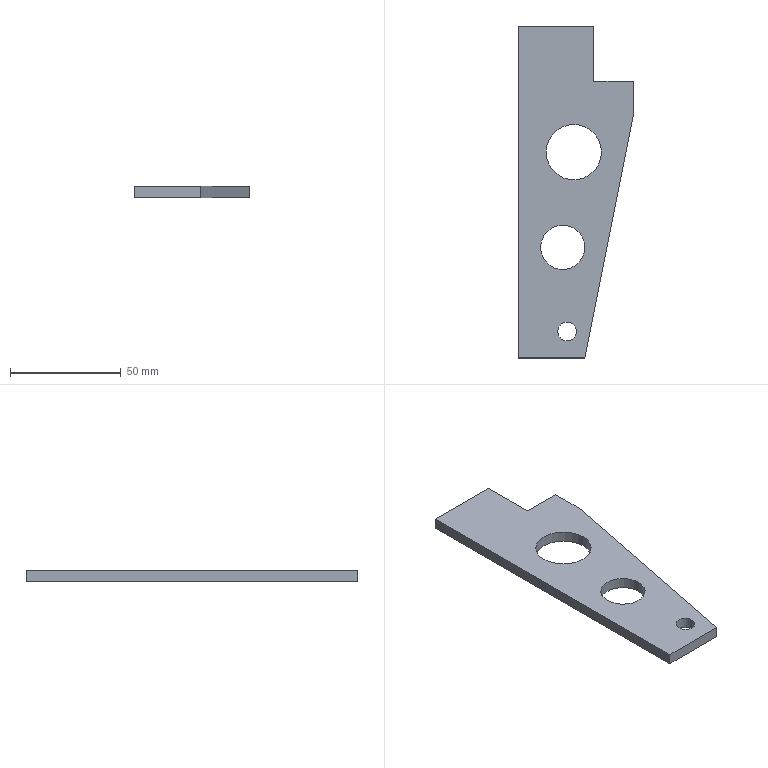Part | NX | features DATUM_CSYS 1, EXTRACT_DATUM_PLANE 1, EXTRUDE 1, SKETCH 1 | 1 solid | 12 faces | box 52 x 150 x 5 mm | volume 26391 mm3 | plane 9 | cylinder 3 | commonest cylinder face diameters 8.5 x1 20 x1 25 x1
STEP:
#1=CARTESIAN_POINT('',(-32.5,57.5,2.5));
#2=VERTEX_POINT('',#1);
#3=CARTESIAN_POINT('',(-32.5,-92.5,2.5));
#4=VERTEX_POINT('',#3);
#5=CARTESIAN_POINT('',(-32.5,57.5,2.5));
#6=DIRECTION('',(0.,-1.,0.));
#7=VECTOR('',#6,1000.);
#8=LINE('',#5,#7);
#9=EDGE_CURVE('',#2,#4,#8,.T.);
#10=ORIENTED_EDGE('',*,*,#9,.F.);
#11=CARTESIAN_POINT('',(-32.5,57.5,-2.5));
#12=VERTEX_POINT('',#11);
#13=CARTESIAN_POINT('',(-32.5,57.5,-2.5));
#14=DIRECTION('',(0.,0.,1.));
#15=VECTOR('',#14,1000.);
#16=LINE('',#13,#15);
#17=EDGE_CURVE('',#12,#2,#16,.T.);
#18=ORIENTED_EDGE('',*,*,#17,.F.);
#19=CARTESIAN_POINT('',(-32.5,-92.5,-2.5));
#20=VERTEX_POINT('',#19);
#21=CARTESIAN_POINT('',(-32.5,57.5,-2.5));
#22=DIRECTION('',(0.,-1.,0.));
#23=VECTOR('',#22,1000.);
#24=LINE('',#21,#23);
#25=EDGE_CURVE('',#12,#20,#24,.T.);
#26=ORIENTED_EDGE('',*,*,#25,.T.);
#27=CARTESIAN_POINT('',(-32.5,-92.5,-2.5));
#28=DIRECTION('',(0.,0.,1.));
#29=VECTOR('',#28,1000.);
#30=LINE('',#27,#29);
#31=EDGE_CURVE('',#20,#4,#30,.T.);
#32=ORIENTED_EDGE('',*,*,#31,.T.);
#33=EDGE_LOOP('',(#10,#18,#26,#32));
#34=FACE_BOUND('',#33,.T.);
#35=CARTESIAN_POINT('',(-32.5,57.5,-2.5));
#36=DIRECTION('',(-1.,0.,0.));
#37=DIRECTION('',(0.,0.,1.));
#38=AXIS2_PLACEMENT_3D('',#35,#36,#37);
#39=PLANE('',#38);
#40=ADVANCED_FACE('',(#34),#39,.T.);
#41=CARTESIAN_POINT('',(-2.5,-92.5,2.5));
#42=VERTEX_POINT('',#41);
#43=CARTESIAN_POINT('',(-32.5,-92.5,2.5));
#44=DIRECTION('',(1.,0.,0.));
#45=VECTOR('',#44,1000.);
#46=LINE('',#43,#45);
#47=EDGE_CURVE('',#4,#42,#46,.T.);
#48=ORIENTED_EDGE('',*,*,#47,.F.);
#49=ORIENTED_EDGE('',*,*,#31,.F.);
#50=CARTESIAN_POINT('',(-2.5,-92.5,-2.5));
#51=VERTEX_POINT('',#50);
#52=CARTESIAN_POINT('',(-32.5,-92.5,-2.5));
#53=DIRECTION('',(1.,0.,0.));
#54=VECTOR('',#53,1000.);
#55=LINE('',#52,#54);
#56=EDGE_CURVE('',#20,#51,#55,.T.);
#57=ORIENTED_EDGE('',*,*,#56,.T.);
#58=CARTESIAN_POINT('',(-2.5,-92.5,-2.5));
#59=DIRECTION('',(0.,0.,1.));
#60=VECTOR('',#59,1000.);
#61=LINE('',#58,#60);
#62=EDGE_CURVE('',#51,#42,#61,.T.);
#63=ORIENTED_EDGE('',*,*,#62,.T.);
#64=EDGE_LOOP('',(#48,#49,#57,#63));
#65=FACE_BOUND('',#64,.T.);
#66=CARTESIAN_POINT('',(-32.5,-92.5,-2.5));
#67=DIRECTION('',(0.,-1.,0.));
#68=DIRECTION('',(0.,0.,-1.));
#69=AXIS2_PLACEMENT_3D('',#66,#67,#68);
#70=PLANE('',#69);
#71=ADVANCED_FACE('',(#65),#70,.T.);
#72=CARTESIAN_POINT('',(19.5,17.5,2.5));
#73=VERTEX_POINT('',#72);
#74=CARTESIAN_POINT('',(-2.5,-92.5,2.5));
#75=DIRECTION('',(0.1961,0.9806,0.));
#76=VECTOR('',#75,1000.);
#77=LINE('',#74,#76);
#78=EDGE_CURVE('',#42,#73,#77,.T.);
#79=ORIENTED_EDGE('',*,*,#78,.F.);
#80=ORIENTED_EDGE('',*,*,#62,.F.);
#81=CARTESIAN_POINT('',(19.5,17.5,-2.5));
#82=VERTEX_POINT('',#81);
#83=CARTESIAN_POINT('',(-2.5,-92.5,-2.5));
#84=DIRECTION('',(0.1961,0.9806,0.));
#85=VECTOR('',#84,1000.);
#86=LINE('',#83,#85);
#87=EDGE_CURVE('',#51,#82,#86,.T.);
#88=ORIENTED_EDGE('',*,*,#87,.T.);
#89=CARTESIAN_POINT('',(19.5,17.5,-2.5));
#90=DIRECTION('',(0.,0.,1.));
#91=VECTOR('',#90,1000.);
#92=LINE('',#89,#91);
#93=EDGE_CURVE('',#82,#73,#92,.T.);
#94=ORIENTED_EDGE('',*,*,#93,.T.);
#95=EDGE_LOOP('',(#79,#80,#88,#94));
#96=FACE_BOUND('',#95,.T.);
#97=CARTESIAN_POINT('',(-2.5,-92.5,-2.5));
#98=DIRECTION('',(0.9806,-0.1961,0.));
#99=DIRECTION('',(0.1961,0.9806,0.));
#100=AXIS2_PLACEMENT_3D('',#97,#98,#99);
#101=PLANE('',#100);
#102=ADVANCED_FACE('',(#96),#101,.T.);
#103=CARTESIAN_POINT('',(19.5,32.5,2.5));
#104=VERTEX_POINT('',#103);
#105=CARTESIAN_POINT('',(19.5,17.5,2.5));
#106=DIRECTION('',(0.,1.,0.));
#107=VECTOR('',#106,1000.);
#108=LINE('',#105,#107);
#109=EDGE_CURVE('',#73,#104,#108,.T.);
#110=ORIENTED_EDGE('',*,*,#109,.F.);
#111=ORIENTED_EDGE('',*,*,#93,.F.);
#112=CARTESIAN_POINT('',(19.5,32.5,-2.5));
#113=VERTEX_POINT('',#112);
#114=CARTESIAN_POINT('',(19.5,17.5,-2.5));
#115=DIRECTION('',(0.,1.,0.));
#116=VECTOR('',#115,1000.);
#117=LINE('',#114,#116);
#118=EDGE_CURVE('',#82,#113,#117,.T.);
#119=ORIENTED_EDGE('',*,*,#118,.T.);
#120=CARTESIAN_POINT('',(19.5,32.5,-2.5));
#121=DIRECTION('',(0.,0.,1.));
#122=VECTOR('',#121,1000.);
#123=LINE('',#120,#122);
#124=EDGE_CURVE('',#113,#104,#123,.T.);
#125=ORIENTED_EDGE('',*,*,#124,.T.);
#126=EDGE_LOOP('',(#110,#111,#119,#125));
#127=FACE_BOUND('',#126,.T.);
#128=CARTESIAN_POINT('',(19.5,17.5,-2.5));
#129=DIRECTION('',(1.,0.,0.));
#130=DIRECTION('',(0.,0.,-1.));
#131=AXIS2_PLACEMENT_3D('',#128,#129,#130);
#132=PLANE('',#131);
#133=ADVANCED_FACE('',(#127),#132,.T.);
#134=CARTESIAN_POINT('',(1.5,32.5,2.5));
#135=VERTEX_POINT('',#134);
#136=CARTESIAN_POINT('',(19.5,32.5,2.5));
#137=DIRECTION('',(-1.,0.,0.));
#138=VECTOR('',#137,1000.);
#139=LINE('',#136,#138);
#140=EDGE_CURVE('',#104,#135,#139,.T.);
#141=ORIENTED_EDGE('',*,*,#140,.F.);
#142=ORIENTED_EDGE('',*,*,#124,.F.);
#143=CARTESIAN_POINT('',(1.5,32.5,-2.5));
#144=VERTEX_POINT('',#143);
#145=CARTESIAN_POINT('',(19.5,32.5,-2.5));
#146=DIRECTION('',(-1.,0.,0.));
#147=VECTOR('',#146,1000.);
#148=LINE('',#145,#147);
#149=EDGE_CURVE('',#113,#144,#148,.T.);
#150=ORIENTED_EDGE('',*,*,#149,.T.);
#151=CARTESIAN_POINT('',(1.5,32.5,-2.5));
#152=DIRECTION('',(0.,0.,1.));
#153=VECTOR('',#152,1000.);
#154=LINE('',#151,#153);
#155=EDGE_CURVE('',#144,#135,#154,.T.);
#156=ORIENTED_EDGE('',*,*,#155,.T.);
#157=EDGE_LOOP('',(#141,#142,#150,#156));
#158=FACE_BOUND('',#157,.T.);
#159=CARTESIAN_POINT('',(19.5,32.5,-2.5));
#160=DIRECTION('',(0.,1.,0.));
#161=DIRECTION('',(0.,0.,1.));
#162=AXIS2_PLACEMENT_3D('',#159,#160,#161);
#163=PLANE('',#162);
#164=ADVANCED_FACE('',(#158),#163,.T.);
#165=CARTESIAN_POINT('',(1.5,57.5,2.5));
#166=VERTEX_POINT('',#165);
#167=CARTESIAN_POINT('',(1.5,32.5,2.5));
#168=DIRECTION('',(0.,1.,0.));
#169=VECTOR('',#168,1000.);
#170=LINE('',#167,#169);
#171=EDGE_CURVE('',#135,#166,#170,.T.);
#172=ORIENTED_EDGE('',*,*,#171,.F.);
#173=ORIENTED_EDGE('',*,*,#155,.F.);
#174=CARTESIAN_POINT('',(1.5,57.5,-2.5));
#175=VERTEX_POINT('',#174);
#176=CARTESIAN_POINT('',(1.5,32.5,-2.5));
#177=DIRECTION('',(0.,1.,0.));
#178=VECTOR('',#177,1000.);
#179=LINE('',#176,#178);
#180=EDGE_CURVE('',#144,#175,#179,.T.);
#181=ORIENTED_EDGE('',*,*,#180,.T.);
#182=CARTESIAN_POINT('',(1.5,57.5,-2.5));
#183=DIRECTION('',(0.,0.,1.));
#184=VECTOR('',#183,1000.);
#185=LINE('',#182,#184);
#186=EDGE_CURVE('',#175,#166,#185,.T.);
#187=ORIENTED_EDGE('',*,*,#186,.T.);
#188=EDGE_LOOP('',(#172,#173,#181,#187));
#189=FACE_BOUND('',#188,.T.);
#190=CARTESIAN_POINT('',(1.5,32.5,-2.5));
#191=DIRECTION('',(1.,0.,0.));
#192=DIRECTION('',(0.,0.,-1.));
#193=AXIS2_PLACEMENT_3D('',#190,#191,#192);
#194=PLANE('',#193);
#195=ADVANCED_FACE('',(#189),#194,.T.);
#196=CARTESIAN_POINT('',(-20.,0.5,2.5));
#197=VERTEX_POINT('',#196);
#198=CARTESIAN_POINT('',(-7.5,0.5,2.5));
#199=DIRECTION('',(0.,0.,-1.));
#200=DIRECTION('',(-1.,0.,0.));
#201=AXIS2_PLACEMENT_3D('',#198,#199,#200);
#202=CIRCLE('',#201,12.5);
#203=EDGE_CURVE('',#197,#197,#202,.T.);
#204=ORIENTED_EDGE('',*,*,#203,.F.);
#205=EDGE_LOOP('',(#204));
#206=FACE_BOUND('',#205,.T.);
#207=CARTESIAN_POINT('',(5.,0.5,-2.5));
#208=VERTEX_POINT('',#207);
#209=CARTESIAN_POINT('',(-7.5,0.5,-2.5));
#210=DIRECTION('',(0.,0.,-1.));
#211=DIRECTION('',(1.,0.,0.));
#212=AXIS2_PLACEMENT_3D('',#209,#210,#211);
#213=CIRCLE('',#212,12.5);
#214=EDGE_CURVE('',#208,#208,#213,.T.);
#215=ORIENTED_EDGE('',*,*,#214,.T.);
#216=EDGE_LOOP('',(#215));
#217=FACE_BOUND('',#216,.T.);
#218=CARTESIAN_POINT('',(-7.5,0.5,-2.5));
#219=DIRECTION('',(0.,0.,1.));
#220=DIRECTION('',(1.,0.,0.));
#221=AXIS2_PLACEMENT_3D('',#218,#219,#220);
#222=CYLINDRICAL_SURFACE('',#221,12.5);
#223=ADVANCED_FACE('',(#206,#217),#222,.F.);
#224=CARTESIAN_POINT('',(-22.5,-42.5,2.5));
#225=VERTEX_POINT('',#224);
#226=CARTESIAN_POINT('',(-12.5,-42.5,2.5));
#227=DIRECTION('',(0.,0.,-1.));
#228=DIRECTION('',(-1.,0.,0.));
#229=AXIS2_PLACEMENT_3D('',#226,#227,#228);
#230=CIRCLE('',#229,10.);
#231=EDGE_CURVE('',#225,#225,#230,.T.);
#232=ORIENTED_EDGE('',*,*,#231,.F.);
#233=EDGE_LOOP('',(#232));
#234=FACE_BOUND('',#233,.T.);
#235=CARTESIAN_POINT('',(-2.5,-42.5,-2.5));
#236=VERTEX_POINT('',#235);
#237=CARTESIAN_POINT('',(-12.5,-42.5,-2.5));
#238=DIRECTION('',(0.,0.,-1.));
#239=DIRECTION('',(1.,0.,0.));
#240=AXIS2_PLACEMENT_3D('',#237,#238,#239);
#241=CIRCLE('',#240,10.);
#242=EDGE_CURVE('',#236,#236,#241,.T.);
#243=ORIENTED_EDGE('',*,*,#242,.T.);
#244=EDGE_LOOP('',(#243));
#245=FACE_BOUND('',#244,.T.);
#246=CARTESIAN_POINT('',(-12.5,-42.5,-2.5));
#247=DIRECTION('',(0.,0.,1.));
#248=DIRECTION('',(1.,0.,0.));
#249=AXIS2_PLACEMENT_3D('',#246,#247,#248);
#250=CYLINDRICAL_SURFACE('',#249,10.);
#251=ADVANCED_FACE('',(#234,#245),#250,.F.);
#252=CARTESIAN_POINT('',(1.5,57.5,2.5));
#253=DIRECTION('',(-1.,0.,0.));
#254=VECTOR('',#253,1000.);
#255=LINE('',#252,#254);
#256=EDGE_CURVE('',#166,#2,#255,.T.);
#257=ORIENTED_EDGE('',*,*,#256,.F.);
#258=ORIENTED_EDGE('',*,*,#186,.F.);
#259=CARTESIAN_POINT('',(1.5,57.5,-2.5));
#260=DIRECTION('',(-1.,0.,0.));
#261=VECTOR('',#260,1000.);
#262=LINE('',#259,#261);
#263=EDGE_CURVE('',#175,#12,#262,.T.);
#264=ORIENTED_EDGE('',*,*,#263,.T.);
#265=ORIENTED_EDGE('',*,*,#17,.T.);
#266=EDGE_LOOP('',(#257,#258,#264,#265));
#267=FACE_BOUND('',#266,.T.);
#268=CARTESIAN_POINT('',(1.5,57.5,-2.5));
#269=DIRECTION('',(0.,1.,0.));
#270=DIRECTION('',(0.,0.,1.));
#271=AXIS2_PLACEMENT_3D('',#268,#269,#270);
#272=PLANE('',#271);
#273=ADVANCED_FACE('',(#267),#272,.T.);
#274=CARTESIAN_POINT('',(-14.75,-80.5,2.5));
#275=VERTEX_POINT('',#274);
#276=CARTESIAN_POINT('',(-10.5,-80.5,2.5));
#277=DIRECTION('',(0.,0.,-1.));
#278=DIRECTION('',(-1.,0.,0.));
#279=AXIS2_PLACEMENT_3D('',#276,#277,#278);
#280=CIRCLE('',#279,4.25);
#281=EDGE_CURVE('',#275,#275,#280,.T.);
#282=ORIENTED_EDGE('',*,*,#281,.F.);
#283=EDGE_LOOP('',(#282));
#284=FACE_BOUND('',#283,.T.);
#285=CARTESIAN_POINT('',(-6.25,-80.5,-2.5));
#286=VERTEX_POINT('',#285);
#287=CARTESIAN_POINT('',(-10.5,-80.5,-2.5));
#288=DIRECTION('',(0.,0.,-1.));
#289=DIRECTION('',(1.,0.,0.));
#290=AXIS2_PLACEMENT_3D('',#287,#288,#289);
#291=CIRCLE('',#290,4.25);
#292=EDGE_CURVE('',#286,#286,#291,.T.);
#293=ORIENTED_EDGE('',*,*,#292,.T.);
#294=EDGE_LOOP('',(#293));
#295=FACE_BOUND('',#294,.T.);
#296=CARTESIAN_POINT('',(-10.5,-80.5,-2.5));
#297=DIRECTION('',(0.,0.,1.));
#298=DIRECTION('',(1.,0.,0.));
#299=AXIS2_PLACEMENT_3D('',#296,#297,#298);
#300=CYLINDRICAL_SURFACE('',#299,4.25);
#301=ADVANCED_FACE('',(#284,#295),#300,.F.);
#302=ORIENTED_EDGE('',*,*,#25,.F.);
#303=ORIENTED_EDGE('',*,*,#263,.F.);
#304=ORIENTED_EDGE('',*,*,#180,.F.);
#305=ORIENTED_EDGE('',*,*,#149,.F.);
#306=ORIENTED_EDGE('',*,*,#118,.F.);
#307=ORIENTED_EDGE('',*,*,#87,.F.);
#308=ORIENTED_EDGE('',*,*,#56,.F.);
#309=EDGE_LOOP('',(#302,#303,#304,#305,#306,#307,#308));
#310=FACE_BOUND('',#309,.T.);
#311=ORIENTED_EDGE('',*,*,#242,.F.);
#312=EDGE_LOOP('',(#311));
#313=FACE_BOUND('',#312,.T.);
#314=ORIENTED_EDGE('',*,*,#214,.F.);
#315=EDGE_LOOP('',(#314));
#316=FACE_BOUND('',#315,.T.);
#317=ORIENTED_EDGE('',*,*,#292,.F.);
#318=EDGE_LOOP('',(#317));
#319=FACE_BOUND('',#318,.T.);
#320=CARTESIAN_POINT('',(-12.5,-42.5,-2.5));
#321=DIRECTION('',(0.,0.,-1.));
#322=DIRECTION('',(-1.,0.,0.));
#323=AXIS2_PLACEMENT_3D('',#320,#321,#322);
#324=PLANE('',#323);
#325=ADVANCED_FACE('',(#310,#313,#316,#319),#324,.T.);
#326=ORIENTED_EDGE('',*,*,#9,.T.);
#327=ORIENTED_EDGE('',*,*,#47,.T.);
#328=ORIENTED_EDGE('',*,*,#78,.T.);
#329=ORIENTED_EDGE('',*,*,#109,.T.);
#330=ORIENTED_EDGE('',*,*,#140,.T.);
#331=ORIENTED_EDGE('',*,*,#171,.T.);
#332=ORIENTED_EDGE('',*,*,#256,.T.);
#333=EDGE_LOOP('',(#326,#327,#328,#329,#330,#331,#332));
#334=FACE_BOUND('',#333,.T.);
#335=ORIENTED_EDGE('',*,*,#231,.T.);
#336=EDGE_LOOP('',(#335));
#337=FACE_BOUND('',#336,.T.);
#338=ORIENTED_EDGE('',*,*,#203,.T.);
#339=EDGE_LOOP('',(#338));
#340=FACE_BOUND('',#339,.T.);
#341=ORIENTED_EDGE('',*,*,#281,.T.);
#342=EDGE_LOOP('',(#341));
#343=FACE_BOUND('',#342,.T.);
#344=CARTESIAN_POINT('',(-12.5,-42.5,2.5));
#345=DIRECTION('',(0.,0.,-1.));
#346=DIRECTION('',(-1.,0.,0.));
#347=AXIS2_PLACEMENT_3D('',#344,#345,#346);
#348=PLANE('',#347);
#349=ADVANCED_FACE('',(#334,#337,#340,#343),#348,.F.);
#350=CLOSED_SHELL('',(#40,#71,#102,#133,#164,#195,#223,#251,#273,#301,#325,#349));
#351=MANIFOLD_SOLID_BREP('',#350);
#352=(LENGTH_UNIT()NAMED_UNIT(*)SI_UNIT(.MILLI.,.METRE.));
#353=UNCERTAINTY_MEASURE_WITH_UNIT(LENGTH_MEASURE(0.00001),#352,'','');
#354=(NAMED_UNIT(*)PLANE_ANGLE_UNIT()SI_UNIT($,.RADIAN.));
#355=(NAMED_UNIT(*)SI_UNIT($,.STERADIAN.)SOLID_ANGLE_UNIT());
#356=(GEOMETRIC_REPRESENTATION_CONTEXT(3)GLOBAL_UNCERTAINTY_ASSIGNED_CONTEXT((#353))GLOBAL_UNIT_ASSIGNED_CONTEXT((#352,#354,#355))REPRESENTATION_CONTEXT('',''));
#357=ADVANCED_BREP_SHAPE_REPRESENTATION('',(#351),#356);